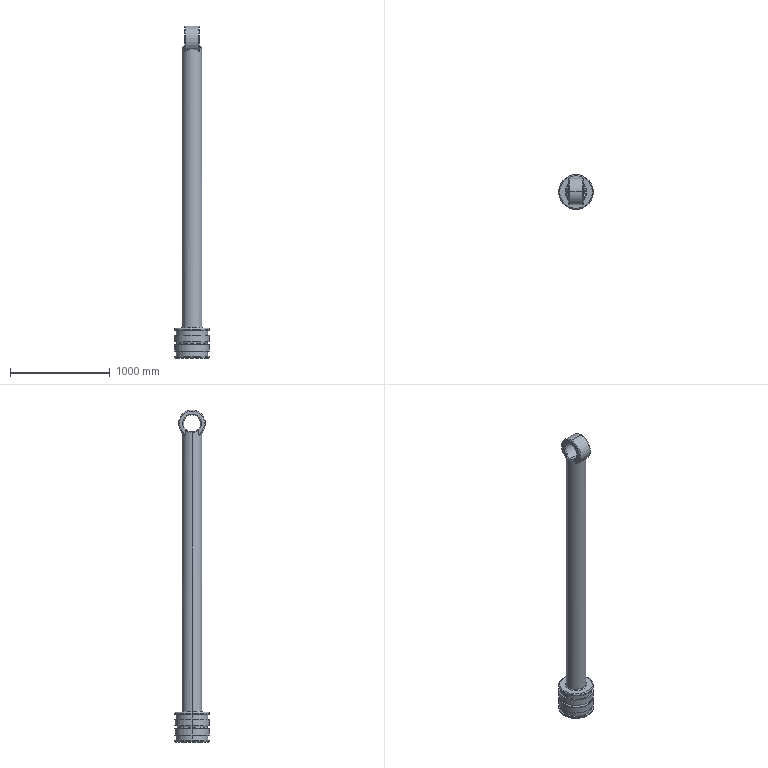Part | SolidWorks | features ICE 4, Fillet 2, RevCut 2, Extrusion 1 | 1 solid | 58 faces | box 349 x 349 x 3335 mm | volume 118986511 mm3 | cylinder 22 | torus 14 | spline 12 | plane 10 | commonest cylinder face diameters 349 x8 20 x4 319 x4 170 x2 200 x2 270.106 x2